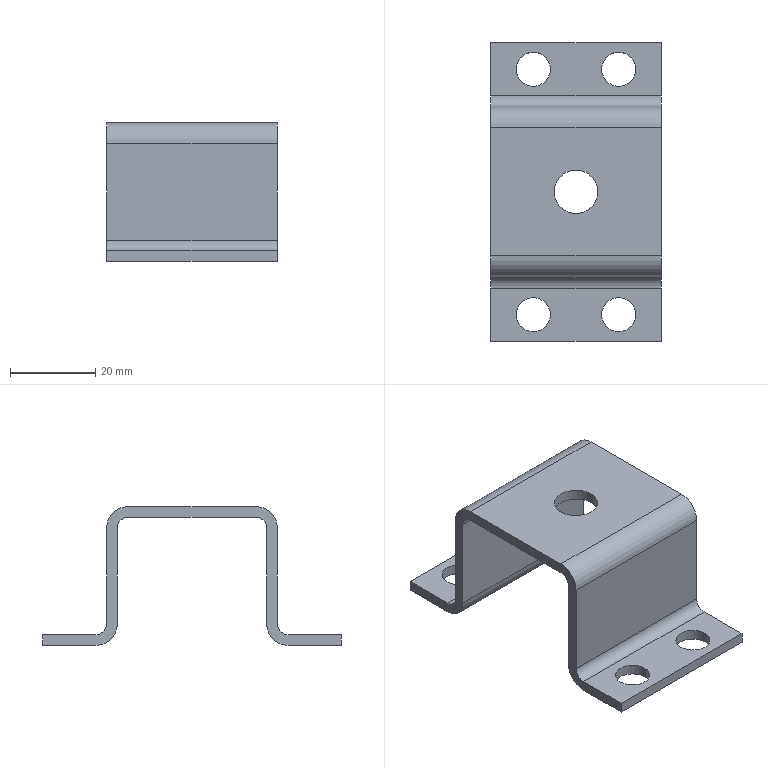Part | NX | features solid 2 | 1 solid | 32 faces | box 40 x 70 x 32.5 mm | volume 11649 mm3 | cylinder 18 | plane 14 | commonest cylinder face diameters 8 x8 5 x4 10 x4 10.2 x2
STEP:
#1=CARTESIAN_POINT('',(-932.,-1394.25,1257.));
#2=VERTEX_POINT('',#1);
#3=CARTESIAN_POINT('',(-932.,-1394.25,1259.5));
#4=VERTEX_POINT('',#3);
#5=CARTESIAN_POINT('',(-932.,-1394.25,1172.573));
#6=DIRECTION('',(0.,0.,1.));
#7=VECTOR('',#6,1000.);
#8=LINE('',#5,#7);
#9=EDGE_CURVE('',#2,#4,#8,.T.);
#10=ORIENTED_EDGE('',*,*,#9,.F.);
#11=CARTESIAN_POINT('',(-924.,-1394.25,1257.));
#12=VERTEX_POINT('',#11);
#13=CARTESIAN_POINT('',(-928.,-1394.25,1257.));
#14=DIRECTION('',(0.,0.,-1.));
#15=DIRECTION('',(0.,1.,0.));
#16=AXIS2_PLACEMENT_3D('',#13,#14,#15);
#17=CIRCLE('',#16,4.);
#18=EDGE_CURVE('',#2,#12,#17,.T.);
#19=ORIENTED_EDGE('',*,*,#18,.T.);
#20=CARTESIAN_POINT('',(-924.,-1394.25,1259.5));
#21=VERTEX_POINT('',#20);
#22=CARTESIAN_POINT('',(-924.,-1394.25,1172.573));
#23=DIRECTION('',(0.,0.,1.));
#24=VECTOR('',#23,1000.);
#25=LINE('',#22,#24);
#26=EDGE_CURVE('',#21,#12,#25,.F.);
#27=ORIENTED_EDGE('',*,*,#26,.F.);
#28=CARTESIAN_POINT('',(-928.,-1394.25,1259.5));
#29=DIRECTION('',(0.,0.,1.));
#30=DIRECTION('',(1.,0.,0.));
#31=AXIS2_PLACEMENT_3D('',#28,#29,#30);
#32=CIRCLE('',#31,4.);
#33=EDGE_CURVE('',#21,#4,#32,.T.);
#34=ORIENTED_EDGE('',*,*,#33,.T.);
#35=EDGE_LOOP('',(#10,#19,#27,#34));
#36=FACE_BOUND('',#35,.T.);
#37=CARTESIAN_POINT('',(-928.,-1394.25,1172.573));
#38=DIRECTION('',(0.,0.,1.));
#39=DIRECTION('',(1.,0.,0.));
#40=AXIS2_PLACEMENT_3D('',#37,#38,#39);
#41=CYLINDRICAL_SURFACE('',#40,4.);
#42=ADVANCED_FACE('',(#36),#41,.F.);
#43=CARTESIAN_POINT('',(-912.,-1394.25,1257.));
#44=VERTEX_POINT('',#43);
#45=CARTESIAN_POINT('',(-912.,-1394.25,1259.5));
#46=VERTEX_POINT('',#45);
#47=CARTESIAN_POINT('',(-912.,-1394.25,1172.573));
#48=DIRECTION('',(0.,0.,1.));
#49=VECTOR('',#48,1000.);
#50=LINE('',#47,#49);
#51=EDGE_CURVE('',#44,#46,#50,.T.);
#52=ORIENTED_EDGE('',*,*,#51,.F.);
#53=CARTESIAN_POINT('',(-904.,-1394.25,1257.));
#54=VERTEX_POINT('',#53);
#55=CARTESIAN_POINT('',(-908.,-1394.25,1257.));
#56=DIRECTION('',(0.,0.,-1.));
#57=DIRECTION('',(0.,1.,0.));
#58=AXIS2_PLACEMENT_3D('',#55,#56,#57);
#59=CIRCLE('',#58,4.);
#60=EDGE_CURVE('',#44,#54,#59,.T.);
#61=ORIENTED_EDGE('',*,*,#60,.T.);
#62=CARTESIAN_POINT('',(-904.,-1394.25,1259.5));
#63=VERTEX_POINT('',#62);
#64=CARTESIAN_POINT('',(-904.,-1394.25,1172.573));
#65=DIRECTION('',(0.,0.,1.));
#66=VECTOR('',#65,1000.);
#67=LINE('',#64,#66);
#68=EDGE_CURVE('',#63,#54,#67,.F.);
#69=ORIENTED_EDGE('',*,*,#68,.F.);
#70=CARTESIAN_POINT('',(-908.,-1394.25,1259.5));
#71=DIRECTION('',(0.,0.,1.));
#72=DIRECTION('',(1.,0.,0.));
#73=AXIS2_PLACEMENT_3D('',#70,#71,#72);
#74=CIRCLE('',#73,4.);
#75=EDGE_CURVE('',#63,#46,#74,.T.);
#76=ORIENTED_EDGE('',*,*,#75,.T.);
#77=EDGE_LOOP('',(#52,#61,#69,#76));
#78=FACE_BOUND('',#77,.T.);
#79=CARTESIAN_POINT('',(-908.,-1394.25,1172.573));
#80=DIRECTION('',(0.,0.,1.));
#81=DIRECTION('',(1.,0.,0.));
#82=AXIS2_PLACEMENT_3D('',#79,#80,#81);
#83=CYLINDRICAL_SURFACE('',#82,4.);
#84=ADVANCED_FACE('',(#78),#83,.F.);
#85=CARTESIAN_POINT('',(-912.,-1451.75,1257.));
#86=VERTEX_POINT('',#85);
#87=CARTESIAN_POINT('',(-912.,-1451.75,1259.5));
#88=VERTEX_POINT('',#87);
#89=CARTESIAN_POINT('',(-912.,-1451.75,1172.573));
#90=DIRECTION('',(0.,0.,1.));
#91=VECTOR('',#90,1000.);
#92=LINE('',#89,#91);
#93=EDGE_CURVE('',#86,#88,#92,.T.);
#94=ORIENTED_EDGE('',*,*,#93,.F.);
#95=CARTESIAN_POINT('',(-904.,-1451.75,1257.));
#96=VERTEX_POINT('',#95);
#97=CARTESIAN_POINT('',(-908.,-1451.75,1257.));
#98=DIRECTION('',(0.,0.,-1.));
#99=DIRECTION('',(-1.,0.,0.));
#100=AXIS2_PLACEMENT_3D('',#97,#98,#99);
#101=CIRCLE('',#100,4.);
#102=EDGE_CURVE('',#86,#96,#101,.T.);
#103=ORIENTED_EDGE('',*,*,#102,.T.);
#104=CARTESIAN_POINT('',(-904.,-1451.75,1259.5));
#105=VERTEX_POINT('',#104);
#106=CARTESIAN_POINT('',(-904.,-1451.75,1172.573));
#107=DIRECTION('',(0.,0.,1.));
#108=VECTOR('',#107,1000.);
#109=LINE('',#106,#108);
#110=EDGE_CURVE('',#105,#96,#109,.F.);
#111=ORIENTED_EDGE('',*,*,#110,.F.);
#112=CARTESIAN_POINT('',(-908.,-1451.75,1259.5));
#113=DIRECTION('',(0.,0.,1.));
#114=DIRECTION('',(1.,0.,0.));
#115=AXIS2_PLACEMENT_3D('',#112,#113,#114);
#116=CIRCLE('',#115,4.);
#117=EDGE_CURVE('',#105,#88,#116,.T.);
#118=ORIENTED_EDGE('',*,*,#117,.T.);
#119=EDGE_LOOP('',(#94,#103,#111,#118));
#120=FACE_BOUND('',#119,.T.);
#121=CARTESIAN_POINT('',(-908.,-1451.75,1172.573));
#122=DIRECTION('',(0.,0.,1.));
#123=DIRECTION('',(1.,0.,0.));
#124=AXIS2_PLACEMENT_3D('',#121,#122,#123);
#125=CYLINDRICAL_SURFACE('',#124,4.);
#126=ADVANCED_FACE('',(#120),#125,.F.);
#127=CARTESIAN_POINT('',(-932.,-1451.75,1257.));
#128=VERTEX_POINT('',#127);
#129=CARTESIAN_POINT('',(-932.,-1451.75,1259.5));
#130=VERTEX_POINT('',#129);
#131=CARTESIAN_POINT('',(-932.,-1451.75,1172.573));
#132=DIRECTION('',(0.,0.,1.));
#133=VECTOR('',#132,1000.);
#134=LINE('',#131,#133);
#135=EDGE_CURVE('',#128,#130,#134,.T.);
#136=ORIENTED_EDGE('',*,*,#135,.F.);
#137=CARTESIAN_POINT('',(-924.,-1451.75,1257.));
#138=VERTEX_POINT('',#137);
#139=CARTESIAN_POINT('',(-928.,-1451.75,1257.));
#140=DIRECTION('',(0.,0.,-1.));
#141=DIRECTION('',(-1.,0.,0.));
#142=AXIS2_PLACEMENT_3D('',#139,#140,#141);
#143=CIRCLE('',#142,4.);
#144=EDGE_CURVE('',#128,#138,#143,.T.);
#145=ORIENTED_EDGE('',*,*,#144,.T.);
#146=CARTESIAN_POINT('',(-924.,-1451.75,1259.5));
#147=VERTEX_POINT('',#146);
#148=CARTESIAN_POINT('',(-924.,-1451.75,1172.573));
#149=DIRECTION('',(0.,0.,1.));
#150=VECTOR('',#149,1000.);
#151=LINE('',#148,#150);
#152=EDGE_CURVE('',#147,#138,#151,.F.);
#153=ORIENTED_EDGE('',*,*,#152,.F.);
#154=CARTESIAN_POINT('',(-928.,-1451.75,1259.5));
#155=DIRECTION('',(0.,0.,1.));
#156=DIRECTION('',(1.,0.,0.));
#157=AXIS2_PLACEMENT_3D('',#154,#155,#156);
#158=CIRCLE('',#157,4.);
#159=EDGE_CURVE('',#147,#130,#158,.T.);
#160=ORIENTED_EDGE('',*,*,#159,.T.);
#161=EDGE_LOOP('',(#136,#145,#153,#160));
#162=FACE_BOUND('',#161,.T.);
#163=CARTESIAN_POINT('',(-928.,-1451.75,1172.573));
#164=DIRECTION('',(0.,0.,1.));
#165=DIRECTION('',(1.,0.,0.));
#166=AXIS2_PLACEMENT_3D('',#163,#164,#165);
#167=CYLINDRICAL_SURFACE('',#166,4.);
#168=ADVANCED_FACE('',(#162),#167,.F.);
#169=CARTESIAN_POINT('',(-923.1,-1423.,1289.5));
#170=VERTEX_POINT('',#169);
#171=CARTESIAN_POINT('',(-923.1,-1423.,1287.));
#172=VERTEX_POINT('',#171);
#173=CARTESIAN_POINT('',(-923.1,-1423.,1202.573));
#174=DIRECTION('',(0.,0.,1.));
#175=VECTOR('',#174,1000.);
#176=LINE('',#173,#175);
#177=EDGE_CURVE('',#170,#172,#176,.F.);
#178=ORIENTED_EDGE('',*,*,#177,.T.);
#179=CARTESIAN_POINT('',(-912.9,-1423.,1287.));
#180=VERTEX_POINT('',#179);
#181=CARTESIAN_POINT('',(-918.,-1423.,1287.));
#182=DIRECTION('',(0.,0.,-1.));
#183=DIRECTION('',(-1.,0.,0.));
#184=AXIS2_PLACEMENT_3D('',#181,#182,#183);
#185=CIRCLE('',#184,5.1);
#186=EDGE_CURVE('',#172,#180,#185,.T.);
#187=ORIENTED_EDGE('',*,*,#186,.T.);
#188=CARTESIAN_POINT('',(-912.9,-1423.,1289.5));
#189=VERTEX_POINT('',#188);
#190=CARTESIAN_POINT('',(-912.9,-1423.,1202.573));
#191=DIRECTION('',(0.,0.,1.));
#192=VECTOR('',#191,1000.);
#193=LINE('',#190,#192);
#194=EDGE_CURVE('',#180,#189,#193,.T.);
#195=ORIENTED_EDGE('',*,*,#194,.T.);
#196=CARTESIAN_POINT('',(-918.,-1423.,1289.5));
#197=DIRECTION('',(0.,0.,1.));
#198=DIRECTION('',(1.,0.,0.));
#199=AXIS2_PLACEMENT_3D('',#196,#197,#198);
#200=CIRCLE('',#199,5.1);
#201=EDGE_CURVE('',#189,#170,#200,.T.);
#202=ORIENTED_EDGE('',*,*,#201,.T.);
#203=EDGE_LOOP('',(#178,#187,#195,#202));
#204=FACE_BOUND('',#203,.T.);
#205=CARTESIAN_POINT('',(-918.,-1423.,1202.573));
#206=DIRECTION('',(0.,0.,1.));
#207=DIRECTION('',(1.,0.,0.));
#208=AXIS2_PLACEMENT_3D('',#205,#206,#207);
#209=CYLINDRICAL_SURFACE('',#208,5.1);
#210=ADVANCED_FACE('',(#204),#209,.F.);
#211=ORIENTED_EDGE('',*,*,#75,.F.);
#212=CARTESIAN_POINT('',(-908.,-1394.25,1259.5));
#213=DIRECTION('',(0.,0.,1.));
#214=DIRECTION('',(1.,0.,0.));
#215=AXIS2_PLACEMENT_3D('',#212,#213,#214);
#216=CIRCLE('',#215,4.);
#217=EDGE_CURVE('',#46,#63,#216,.T.);
#218=ORIENTED_EDGE('',*,*,#217,.F.);
#219=EDGE_LOOP('',(#211,#218));
#220=FACE_BOUND('',#219,.T.);
#221=ORIENTED_EDGE('',*,*,#33,.F.);
#222=CARTESIAN_POINT('',(-928.,-1394.25,1259.5));
#223=DIRECTION('',(0.,0.,1.));
#224=DIRECTION('',(1.,0.,0.));
#225=AXIS2_PLACEMENT_3D('',#222,#223,#224);
#226=CIRCLE('',#225,4.);
#227=EDGE_CURVE('',#4,#21,#226,.T.);
#228=ORIENTED_EDGE('',*,*,#227,.F.);
#229=EDGE_LOOP('',(#221,#228));
#230=FACE_BOUND('',#229,.T.);
#231=CARTESIAN_POINT('',(-898.,-1400.5,1259.5));
#232=VERTEX_POINT('',#231);
#233=CARTESIAN_POINT('',(-898.,-1388.,1259.5));
#234=VERTEX_POINT('',#233);
#235=CARTESIAN_POINT('',(-898.,-1403.,1259.5));
#236=DIRECTION('',(0.,1.,0.));
#237=VECTOR('',#236,1000.);
#238=LINE('',#235,#237);
#239=EDGE_CURVE('',#232,#234,#238,.T.);
#240=ORIENTED_EDGE('',*,*,#239,.T.);
#241=CARTESIAN_POINT('',(-938.,-1388.,1259.5));
#242=VERTEX_POINT('',#241);
#243=CARTESIAN_POINT('',(-938.,-1388.,1259.5));
#244=DIRECTION('',(1.,0.,0.));
#245=VECTOR('',#244,1000.);
#246=LINE('',#243,#245);
#247=EDGE_CURVE('',#242,#234,#246,.T.);
#248=ORIENTED_EDGE('',*,*,#247,.F.);
#249=CARTESIAN_POINT('',(-938.,-1400.5,1259.5));
#250=VERTEX_POINT('',#249);
#251=CARTESIAN_POINT('',(-938.,-1403.,1259.5));
#252=DIRECTION('',(0.,1.,0.));
#253=VECTOR('',#252,1000.);
#254=LINE('',#251,#253);
#255=EDGE_CURVE('',#250,#242,#254,.T.);
#256=ORIENTED_EDGE('',*,*,#255,.F.);
#257=CARTESIAN_POINT('',(-938.,-1400.5,1259.5));
#258=DIRECTION('',(1.,0.,0.));
#259=VECTOR('',#258,1000.);
#260=LINE('',#257,#259);
#261=EDGE_CURVE('',#250,#232,#260,.T.);
#262=ORIENTED_EDGE('',*,*,#261,.T.);
#263=EDGE_LOOP('',(#240,#248,#256,#262));
#264=FACE_BOUND('',#263,.T.);
#265=CARTESIAN_POINT('',(-938.,-1403.,1259.5));
#266=DIRECTION('',(0.,0.,-1.));
#267=DIRECTION('',(0.,-1.,0.));
#268=AXIS2_PLACEMENT_3D('',#265,#266,#267);
#269=PLANE('',#268);
#270=ADVANCED_FACE('',(#220,#230,#264),#269,.F.);
#271=CARTESIAN_POINT('',(-898.,-1403.,1262.));
#272=VERTEX_POINT('',#271);
#273=CARTESIAN_POINT('',(-898.,-1400.5,1262.));
#274=DIRECTION('',(1.,0.,0.));
#275=DIRECTION('',(0.,-1.,0.));
#276=AXIS2_PLACEMENT_3D('',#273,#274,#275);
#277=CIRCLE('',#276,2.5);
#278=EDGE_CURVE('',#272,#232,#277,.T.);
#279=ORIENTED_EDGE('',*,*,#278,.T.);
#280=ORIENTED_EDGE('',*,*,#261,.F.);
#281=CARTESIAN_POINT('',(-938.,-1403.,1262.));
#282=VERTEX_POINT('',#281);
#283=CARTESIAN_POINT('',(-938.,-1400.5,1262.));
#284=DIRECTION('',(1.,0.,0.));
#285=DIRECTION('',(0.,-1.,0.));
#286=AXIS2_PLACEMENT_3D('',#283,#284,#285);
#287=CIRCLE('',#286,2.5);
#288=EDGE_CURVE('',#282,#250,#287,.T.);
#289=ORIENTED_EDGE('',*,*,#288,.F.);
#290=CARTESIAN_POINT('',(-938.,-1403.,1262.));
#291=DIRECTION('',(1.,0.,0.));
#292=VECTOR('',#291,1000.);
#293=LINE('',#290,#292);
#294=EDGE_CURVE('',#282,#272,#293,.T.);
#295=ORIENTED_EDGE('',*,*,#294,.T.);
#296=EDGE_LOOP('',(#279,#280,#289,#295));
#297=FACE_BOUND('',#296,.T.);
#298=CARTESIAN_POINT('',(-938.,-1400.5,1262.));
#299=DIRECTION('',(1.,0.,0.));
#300=DIRECTION('',(0.,0.,-1.));
#301=AXIS2_PLACEMENT_3D('',#298,#299,#300);
#302=CYLINDRICAL_SURFACE('',#301,2.5);
#303=ADVANCED_FACE('',(#297),#302,.F.);
#304=CARTESIAN_POINT('',(-898.,-1403.,1284.5));
#305=VERTEX_POINT('',#304);
#306=CARTESIAN_POINT('',(-898.,-1403.,1289.5));
#307=DIRECTION('',(0.,0.,-1.));
#308=VECTOR('',#307,1000.);
#309=LINE('',#306,#308);
#310=EDGE_CURVE('',#305,#272,#309,.T.);
#311=ORIENTED_EDGE('',*,*,#310,.T.);
#312=ORIENTED_EDGE('',*,*,#294,.F.);
#313=CARTESIAN_POINT('',(-938.,-1403.,1284.5));
#314=VERTEX_POINT('',#313);
#315=CARTESIAN_POINT('',(-938.,-1403.,1289.5));
#316=DIRECTION('',(0.,0.,-1.));
#317=VECTOR('',#316,1000.);
#318=LINE('',#315,#317);
#319=EDGE_CURVE('',#314,#282,#318,.T.);
#320=ORIENTED_EDGE('',*,*,#319,.F.);
#321=CARTESIAN_POINT('',(-938.,-1403.,1284.5));
#322=DIRECTION('',(1.,0.,0.));
#323=VECTOR('',#322,1000.);
#324=LINE('',#321,#323);
#325=EDGE_CURVE('',#314,#305,#324,.T.);
#326=ORIENTED_EDGE('',*,*,#325,.T.);
#327=EDGE_LOOP('',(#311,#312,#320,#326));
#328=FACE_BOUND('',#327,.T.);
#329=CARTESIAN_POINT('',(-938.,-1403.,1289.5));
#330=DIRECTION('',(0.,-1.,0.));
#331=DIRECTION('',(0.,0.,-1.));
#332=AXIS2_PLACEMENT_3D('',#329,#330,#331);
#333=PLANE('',#332);
#334=ADVANCED_FACE('',(#328),#333,.F.);
#335=CARTESIAN_POINT('',(-898.,-1408.,1289.5));
#336=VERTEX_POINT('',#335);
#337=CARTESIAN_POINT('',(-898.,-1408.,1284.5));
#338=DIRECTION('',(-1.,0.,0.));
#339=DIRECTION('',(0.,1.,0.));
#340=AXIS2_PLACEMENT_3D('',#337,#338,#339);
#341=CIRCLE('',#340,5.);
#342=EDGE_CURVE('',#336,#305,#341,.T.);
#343=ORIENTED_EDGE('',*,*,#342,.T.);
#344=ORIENTED_EDGE('',*,*,#325,.F.);
#345=CARTESIAN_POINT('',(-938.,-1408.,1289.5));
#346=VERTEX_POINT('',#345);
#347=CARTESIAN_POINT('',(-938.,-1408.,1284.5));
#348=DIRECTION('',(-1.,0.,0.));
#349=DIRECTION('',(0.,1.,0.));
#350=AXIS2_PLACEMENT_3D('',#347,#348,#349);
#351=CIRCLE('',#350,5.);
#352=EDGE_CURVE('',#346,#314,#351,.T.);
#353=ORIENTED_EDGE('',*,*,#352,.F.);
#354=CARTESIAN_POINT('',(-938.,-1408.,1289.5));
#355=DIRECTION('',(1.,0.,0.));
#356=VECTOR('',#355,1000.);
#357=LINE('',#354,#356);
#358=EDGE_CURVE('',#346,#336,#357,.T.);
#359=ORIENTED_EDGE('',*,*,#358,.T.);
#360=EDGE_LOOP('',(#343,#344,#353,#359));
#361=FACE_BOUND('',#360,.T.);
#362=CARTESIAN_POINT('',(-938.,-1408.,1284.5));
#363=DIRECTION('',(1.,0.,0.));
#364=DIRECTION('',(0.,0.,-1.));
#365=AXIS2_PLACEMENT_3D('',#362,#363,#364);
#366=CYLINDRICAL_SURFACE('',#365,5.);
#367=ADVANCED_FACE('',(#361),#366,.T.);
#368=ORIENTED_EDGE('',*,*,#201,.F.);
#369=CARTESIAN_POINT('',(-918.,-1423.,1289.5));
#370=DIRECTION('',(0.,0.,1.));
#371=DIRECTION('',(1.,0.,0.));
#372=AXIS2_PLACEMENT_3D('',#369,#370,#371);
#373=CIRCLE('',#372,5.1);
#374=EDGE_CURVE('',#170,#189,#373,.T.);
#375=ORIENTED_EDGE('',*,*,#374,.F.);
#376=EDGE_LOOP('',(#368,#375));
#377=FACE_BOUND('',#376,.T.);
#378=CARTESIAN_POINT('',(-898.,-1438.,1289.5));
#379=VERTEX_POINT('',#378);
#380=CARTESIAN_POINT('',(-898.,-1443.,1289.5));
#381=DIRECTION('',(0.,1.,0.));
#382=VECTOR('',#381,1000.);
#383=LINE('',#380,#382);
#384=EDGE_CURVE('',#379,#336,#383,.T.);
#385=ORIENTED_EDGE('',*,*,#384,.T.);
#386=ORIENTED_EDGE('',*,*,#358,.F.);
#387=CARTESIAN_POINT('',(-938.,-1438.,1289.5));
#388=VERTEX_POINT('',#387);
#389=CARTESIAN_POINT('',(-938.,-1443.,1289.5));
#390=DIRECTION('',(0.,1.,0.));
#391=VECTOR('',#390,1000.);
#392=LINE('',#389,#391);
#393=EDGE_CURVE('',#388,#346,#392,.T.);
#394=ORIENTED_EDGE('',*,*,#393,.F.);
#395=CARTESIAN_POINT('',(-938.,-1438.,1289.5));
#396=DIRECTION('',(1.,0.,0.));
#397=VECTOR('',#396,1000.);
#398=LINE('',#395,#397);
#399=EDGE_CURVE('',#388,#379,#398,.T.);
#400=ORIENTED_EDGE('',*,*,#399,.T.);
#401=EDGE_LOOP('',(#385,#386,#394,#400));
#402=FACE_BOUND('',#401,.T.);
#403=CARTESIAN_POINT('',(-938.,-1443.,1289.5));
#404=DIRECTION('',(0.,0.,-1.));
#405=DIRECTION('',(0.,-1.,0.));
#406=AXIS2_PLACEMENT_3D('',#403,#404,#405);
#407=PLANE('',#406);
#408=ADVANCED_FACE('',(#377,#402),#407,.F.);
#409=CARTESIAN_POINT('',(-898.,-1443.,1284.5));
#410=VERTEX_POINT('',#409);
#411=CARTESIAN_POINT('',(-898.,-1438.,1284.5));
#412=DIRECTION('',(-1.,0.,0.));
#413=DIRECTION('',(0.,1.,0.));
#414=AXIS2_PLACEMENT_3D('',#411,#412,#413);
#415=CIRCLE('',#414,5.);
#416=EDGE_CURVE('',#410,#379,#415,.T.);
#417=ORIENTED_EDGE('',*,*,#416,.T.);
#418=ORIENTED_EDGE('',*,*,#399,.F.);
#419=CARTESIAN_POINT('',(-938.,-1443.,1284.5));
#420=VERTEX_POINT('',#419);
#421=CARTESIAN_POINT('',(-938.,-1438.,1284.5));
#422=DIRECTION('',(-1.,0.,0.));
#423=DIRECTION('',(0.,1.,0.));
#424=AXIS2_PLACEMENT_3D('',#421,#422,#423);
#425=CIRCLE('',#424,5.);
#426=EDGE_CURVE('',#420,#388,#425,.T.);
#427=ORIENTED_EDGE('',*,*,#426,.F.);
#428=CARTESIAN_POINT('',(-938.,-1443.,1284.5));
#429=DIRECTION('',(1.,0.,0.));
#430=VECTOR('',#429,1000.);
#431=LINE('',#428,#430);
#432=EDGE_CURVE('',#420,#410,#431,.T.);
#433=ORIENTED_EDGE('',*,*,#432,.T.);
#434=EDGE_LOOP('',(#417,#418,#427,#433));
#435=FACE_BOUND('',#434,.T.);
#436=CARTESIAN_POINT('',(-938.,-1438.,1284.5));
#437=DIRECTION('',(1.,0.,0.));
#438=DIRECTION('',(0.,0.,-1.));
#439=AXIS2_PLACEMENT_3D('',#436,#437,#438);
#440=CYLINDRICAL_SURFACE('',#439,5.);
#441=ADVANCED_FACE('',(#435),#440,.T.);
#442=CARTESIAN_POINT('',(-898.,-1443.,1262.));
#443=VERTEX_POINT('',#442);
#444=CARTESIAN_POINT('',(-898.,-1443.,1259.5));
#445=DIRECTION('',(0.,0.,1.));
#446=VECTOR('',#445,1000.);
#447=LINE('',#444,#446);
#448=EDGE_CURVE('',#443,#410,#447,.T.);
#449=ORIENTED_EDGE('',*,*,#448,.T.);
#450=ORIENTED_EDGE('',*,*,#432,.F.);
#451=CARTESIAN_POINT('',(-938.,-1443.,1262.));
#452=VERTEX_POINT('',#451);
#453=CARTESIAN_POINT('',(-938.,-1443.,1259.5));
#454=DIRECTION('',(0.,0.,1.));
#455=VECTOR('',#454,1000.);
#456=LINE('',#453,#455);
#457=EDGE_CURVE('',#452,#420,#456,.T.);
#458=ORIENTED_EDGE('',*,*,#457,.F.);
#459=CARTESIAN_POINT('',(-938.,-1443.,1262.));
#460=DIRECTION('',(1.,0.,0.));
#461=VECTOR('',#460,1000.);
#462=LINE('',#459,#461);
#463=EDGE_CURVE('',#452,#443,#462,.T.);
#464=ORIENTED_EDGE('',*,*,#463,.T.);
#465=EDGE_LOOP('',(#449,#450,#458,#464));
#466=FACE_BOUND('',#465,.T.);
#467=CARTESIAN_POINT('',(-938.,-1443.,1259.5));
#468=DIRECTION('',(0.,1.,0.));
#469=DIRECTION('',(0.,0.,-1.));
#470=AXIS2_PLACEMENT_3D('',#467,#468,#469);
#471=PLANE('',#470);
#472=ADVANCED_FACE('',(#466),#471,.F.);
#473=CARTESIAN_POINT('',(-898.,-1445.5,1259.5));
#474=VERTEX_POINT('',#473);
#475=CARTESIAN_POINT('',(-898.,-1445.5,1262.));
#476=DIRECTION('',(1.,0.,0.));
#477=DIRECTION('',(0.,-1.,0.));
#478=AXIS2_PLACEMENT_3D('',#475,#476,#477);
#479=CIRCLE('',#478,2.5);
#480=EDGE_CURVE('',#474,#443,#479,.T.);
#481=ORIENTED_EDGE('',*,*,#480,.T.);
#482=ORIENTED_EDGE('',*,*,#463,.F.);
#483=CARTESIAN_POINT('',(-938.,-1445.5,1259.5));
#484=VERTEX_POINT('',#483);
#485=CARTESIAN_POINT('',(-938.,-1445.5,1262.));
#486=DIRECTION('',(1.,0.,0.));
#487=DIRECTION('',(0.,-1.,0.));
#488=AXIS2_PLACEMENT_3D('',#485,#486,#487);
#489=CIRCLE('',#488,2.5);
#490=EDGE_CURVE('',#484,#452,#489,.T.);
#491=ORIENTED_EDGE('',*,*,#490,.F.);
#492=CARTESIAN_POINT('',(-938.,-1445.5,1259.5));
#493=DIRECTION('',(1.,0.,0.));
#494=VECTOR('',#493,1000.);
#495=LINE('',#492,#494);
#496=EDGE_CURVE('',#484,#474,#495,.T.);
#497=ORIENTED_EDGE('',*,*,#496,.T.);
#498=EDGE_LOOP('',(#481,#482,#491,#497));
#499=FACE_BOUND('',#498,.T.);
#500=CARTESIAN_POINT('',(-938.,-1445.5,1262.));
#501=DIRECTION('',(1.,0.,0.));
#502=DIRECTION('',(0.,0.,-1.));
#503=AXIS2_PLACEMENT_3D('',#500,#501,#502);
#504=CYLINDRICAL_SURFACE('',#503,2.5);
#505=ADVANCED_FACE('',(#499),#504,.F.);
#506=ORIENTED_EDGE('',*,*,#159,.F.);
#507=CARTESIAN_POINT('',(-928.,-1451.75,1259.5));
#508=DIRECTION('',(0.,0.,1.));
#509=DIRECTION('',(1.,0.,0.));
#510=AXIS2_PLACEMENT_3D('',#507,#508,#509);
#511=CIRCLE('',#510,4.);
#512=EDGE_CURVE('',#130,#147,#511,.T.);
#513=ORIENTED_EDGE('',*,*,#512,.F.);
#514=EDGE_LOOP('',(#506,#513));
#515=FACE_BOUND('',#514,.T.);
#516=ORIENTED_EDGE('',*,*,#117,.F.);
#517=CARTESIAN_POINT('',(-908.,-1451.75,1259.5));
#518=DIRECTION('',(0.,0.,1.));
#519=DIRECTION('',(1.,0.,0.));
#520=AXIS2_PLACEMENT_3D('',#517,#518,#519);
#521=CIRCLE('',#520,4.);
#522=EDGE_CURVE('',#88,#105,#521,.T.);
#523=ORIENTED_EDGE('',*,*,#522,.F.);
#524=EDGE_LOOP('',(#516,#523));
#525=FACE_BOUND('',#524,.T.);
#526=CARTESIAN_POINT('',(-898.,-1458.,1259.5));
#527=VERTEX_POINT('',#526);
#528=CARTESIAN_POINT('',(-898.,-1458.,1259.5));
#529=DIRECTION('',(0.,1.,0.));
#530=VECTOR('',#529,1000.);
#531=LINE('',#528,#530);
#532=EDGE_CURVE('',#527,#474,#531,.T.);
#533=ORIENTED_EDGE('',*,*,#532,.T.);
#534=ORIENTED_EDGE('',*,*,#496,.F.);
#535=CARTESIAN_POINT('',(-938.,-1458.,1259.5));
#536=VERTEX_POINT('',#535);
#537=CARTESIAN_POINT('',(-938.,-1458.,1259.5));
#538=DIRECTION('',(0.,1.,0.));
#539=VECTOR('',#538,1000.);
#540=LINE('',#537,#539);
#541=EDGE_CURVE('',#536,#484,#540,.T.);
#542=ORIENTED_EDGE('',*,*,#541,.F.);
#543=CARTESIAN_POINT('',(-938.,-1458.,1259.5));
#544=DIRECTION('',(1.,0.,0.));
#545=VECTOR('',#544,1000.);
#546=LINE('',#543,#545);
#547=EDGE_CURVE('',#536,#527,#546,.T.);
#548=ORIENTED_EDGE('',*,*,#547,.T.);
#549=EDGE_LOOP('',(#533,#534,#542,#548));
#550=FACE_BOUND('',#549,.T.);
#551=CARTESIAN_POINT('',(-938.,-1458.,1259.5));
#552=DIRECTION('',(0.,0.,-1.));
#553=DIRECTION('',(0.,-1.,0.));
#554=AXIS2_PLACEMENT_3D('',#551,#552,#553);
#555=PLANE('',#554);
#556=ADVANCED_FACE('',(#515,#525,#550),#555,.F.);
#557=CARTESIAN_POINT('',(-908.,-1394.25,1257.));
#558=DIRECTION('',(0.,0.,-1.));
#559=DIRECTION('',(0.,1.,0.));
#560=AXIS2_PLACEMENT_3D('',#557,#558,#559);
#561=CIRCLE('',#560,4.);
#562=EDGE_CURVE('',#54,#44,#561,.T.);
#563=ORIENTED_EDGE('',*,*,#562,.F.);
#564=ORIENTED_EDGE('',*,*,#60,.F.);
#565=EDGE_LOOP('',(#563,#564));
#566=FACE_BOUND('',#565,.T.);
#567=CARTESIAN_POINT('',(-928.,-1394.25,1257.));
#568=DIRECTION('',(0.,0.,-1.));
#569=DIRECTION('',(0.,1.,0.));
#570=AXIS2_PLACEMENT_3D('',#567,#568,#569);
#571=CIRCLE('',#570,4.);
#572=EDGE_CURVE('',#12,#2,#571,.T.);
#573=ORIENTED_EDGE('',*,*,#572,.F.);
#574=ORIENTED_EDGE('',*,*,#18,.F.);
#575=EDGE_LOOP('',(#573,#574));
#576=FACE_BOUND('',#575,.T.);
#577=CARTESIAN_POINT('',(-898.,-1400.5,1257.));
#578=VERTEX_POINT('',#577);
#579=CARTESIAN_POINT('',(-898.,-1388.,1257.));
#580=VERTEX_POINT('',#579);
#581=CARTESIAN_POINT('',(-898.,-1403.,1257.));
#582=DIRECTION('',(0.,1.,0.));
#583=VECTOR('',#582,1000.);
#584=LINE('',#581,#583);
#585=EDGE_CURVE('',#578,#580,#584,.T.);
#586=ORIENTED_EDGE('',*,*,#585,.F.);
#587=CARTESIAN_POINT('',(-938.,-1400.5,1257.));
#588=VERTEX_POINT('',#587);
#589=CARTESIAN_POINT('',(-938.,-1400.5,1257.));
#590=DIRECTION('',(1.,0.,0.));
#591=VECTOR('',#590,1000.);
#592=LINE('',#589,#591);
#593=EDGE_CURVE('',#588,#578,#592,.T.);
#594=ORIENTED_EDGE('',*,*,#593,.F.);
#595=CARTESIAN_POINT('',(-938.,-1388.,1257.));
#596=VERTEX_POINT('',#595);
#597=CARTESIAN_POINT('',(-938.,-1403.,1257.));
#598=DIRECTION('',(0.,1.,0.));
#599=VECTOR('',#598,1000.);
#600=LINE('',#597,#599);
#601=EDGE_CURVE('',#588,#596,#600,.T.);
#602=ORIENTED_EDGE('',*,*,#601,.T.);
#603=CARTESIAN_POINT('',(-938.,-1388.,1257.));
#604=DIRECTION('',(1.,0.,0.));
#605=VECTOR('',#604,1000.);
#606=LINE('',#603,#605);
#607=EDGE_CURVE('',#596,#580,#606,.T.);
#608=ORIENTED_EDGE('',*,*,#607,.T.);
#609=EDGE_LOOP('',(#586,#594,#602,#608));
#610=FACE_BOUND('',#609,.T.);
#611=CARTESIAN_POINT('',(-938.,-1403.,1257.));
#612=DIRECTION('',(0.,0.,-1.));
#613=DIRECTION('',(0.,-1.,0.));
#614=AXIS2_PLACEMENT_3D('',#611,#612,#613);
#615=PLANE('',#614);
#616=ADVANCED_FACE('',(#566,#576,#610),#615,.T.);
#617=CARTESIAN_POINT('',(-898.,-1405.5,1262.));
#618=VERTEX_POINT('',#617);
#619=CARTESIAN_POINT('',(-898.,-1400.5,1262.));
#620=DIRECTION('',(1.,0.,0.));
#621=DIRECTION('',(0.,0.,-1.));
#622=AXIS2_PLACEMENT_3D('',#619,#620,#621);
#623=CIRCLE('',#622,5.);
#624=EDGE_CURVE('',#618,#578,#623,.T.);
#625=ORIENTED_EDGE('',*,*,#624,.F.);
#626=CARTESIAN_POINT('',(-938.,-1405.5,1262.));
#627=VERTEX_POINT('',#626);
#628=CARTESIAN_POINT('',(-938.,-1405.5,1262.));
#629=DIRECTION('',(1.,0.,0.));
#630=VECTOR('',#629,1000.);
#631=LINE('',#628,#630);
#632=EDGE_CURVE('',#627,#618,#631,.T.);
#633=ORIENTED_EDGE('',*,*,#632,.F.);
#634=CARTESIAN_POINT('',(-938.,-1400.5,1262.));
#635=DIRECTION('',(1.,0.,0.));
#636=DIRECTION('',(0.,0.,-1.));
#637=AXIS2_PLACEMENT_3D('',#634,#635,#636);
#638=CIRCLE('',#637,5.);
#639=EDGE_CURVE('',#627,#588,#638,.T.);
#640=ORIENTED_EDGE('',*,*,#639,.T.);
#641=ORIENTED_EDGE('',*,*,#593,.T.);
#642=EDGE_LOOP('',(#625,#633,#640,#641));
#643=FACE_BOUND('',#642,.T.);
#644=CARTESIAN_POINT('',(-938.,-1400.5,1262.));
#645=DIRECTION('',(1.,0.,0.));
#646=DIRECTION('',(0.,0.,-1.));
#647=AXIS2_PLACEMENT_3D('',#644,#645,#646);
#648=CYLINDRICAL_SURFACE('',#647,5.);
#649=ADVANCED_FACE('',(#643),#648,.T.);
#650=CARTESIAN_POINT('',(-898.,-1405.5,1284.5));
#651=VERTEX_POINT('',#650);
#652=CARTESIAN_POINT('',(-898.,-1405.5,1289.5));
#653=DIRECTION('',(0.,0.,-1.));
#654=VECTOR('',#653,1000.);
#655=LINE('',#652,#654);
#656=EDGE_CURVE('',#651,#618,#655,.T.);
#657=ORIENTED_EDGE('',*,*,#656,.F.);
#658=CARTESIAN_POINT('',(-938.,-1405.5,1284.5));
#659=VERTEX_POINT('',#658);
#660=CARTESIAN_POINT('',(-938.,-1405.5,1284.5));
#661=DIRECTION('',(1.,0.,0.));
#662=VECTOR('',#661,1000.);
#663=LINE('',#660,#662);
#664=EDGE_CURVE('',#659,#651,#663,.T.);
#665=ORIENTED_EDGE('',*,*,#664,.F.);
#666=CARTESIAN_POINT('',(-938.,-1405.5,1289.5));
#667=DIRECTION('',(0.,0.,-1.));
#668=VECTOR('',#667,1000.);
#669=LINE('',#666,#668);
#670=EDGE_CURVE('',#659,#627,#669,.T.);
#671=ORIENTED_EDGE('',*,*,#670,.T.);
#672=ORIENTED_EDGE('',*,*,#632,.T.);
#673=EDGE_LOOP('',(#657,#665,#671,#672));
#674=FACE_BOUND('',#673,.T.);
#675=CARTESIAN_POINT('',(-938.,-1405.5,1289.5));
#676=DIRECTION('',(0.,-1.,0.));
#677=DIRECTION('',(0.,0.,-1.));
#678=AXIS2_PLACEMENT_3D('',#675,#676,#677);
#679=PLANE('',#678);
#680=ADVANCED_FACE('',(#674),#679,.T.);
#681=CARTESIAN_POINT('',(-898.,-1408.,1287.));
#682=VERTEX_POINT('',#681);
#683=CARTESIAN_POINT('',(-898.,-1408.,1284.5));
#684=DIRECTION('',(-1.,0.,0.));
#685=DIRECTION('',(0.,0.,-1.));
#686=AXIS2_PLACEMENT_3D('',#683,#684,#685);
#687=CIRCLE('',#686,2.5);
#688=EDGE_CURVE('',#682,#651,#687,.T.);
#689=ORIENTED_EDGE('',*,*,#688,.F.);
#690=CARTESIAN_POINT('',(-938.,-1408.,1287.));
#691=VERTEX_POINT('',#690);
#692=CARTESIAN_POINT('',(-938.,-1408.,1287.));
#693=DIRECTION('',(1.,0.,0.));
#694=VECTOR('',#693,1000.);
#695=LINE('',#692,#694);
#696=EDGE_CURVE('',#691,#682,#695,.T.);
#697=ORIENTED_EDGE('',*,*,#696,.F.);
#698=CARTESIAN_POINT('',(-938.,-1408.,1284.5));
#699=DIRECTION('',(-1.,0.,0.));
#700=DIRECTION('',(0.,0.,-1.));
#701=AXIS2_PLACEMENT_3D('',#698,#699,#700);
#702=CIRCLE('',#701,2.5);
#703=EDGE_CURVE('',#691,#659,#702,.T.);
#704=ORIENTED_EDGE('',*,*,#703,.T.);
#705=ORIENTED_EDGE('',*,*,#664,.T.);
#706=EDGE_LOOP('',(#689,#697,#704,#705));
#707=FACE_BOUND('',#706,.T.);
#708=CARTESIAN_POINT('',(-938.,-1408.,1284.5));
#709=DIRECTION('',(1.,0.,0.));
#710=DIRECTION('',(0.,0.,-1.));
#711=AXIS2_PLACEMENT_3D('',#708,#709,#710);
#712=CYLINDRICAL_SURFACE('',#711,2.5);
#713=ADVANCED_FACE('',(#707),#712,.F.);
#714=CARTESIAN_POINT('',(-918.,-1423.,1287.));
#715=DIRECTION('',(0.,0.,-1.));
#716=DIRECTION('',(-1.,0.,0.));
#717=AXIS2_PLACEMENT_3D('',#714,#715,#716);
#718=CIRCLE('',#717,5.1);
#719=EDGE_CURVE('',#180,#172,#718,.T.);
#720=ORIENTED_EDGE('',*,*,#719,.F.);
#721=ORIENTED_EDGE('',*,*,#186,.F.);
#722=EDGE_LOOP('',(#720,#721));
#723=FACE_BOUND('',#722,.T.);
#724=CARTESIAN_POINT('',(-898.,-1438.,1287.));
#725=VERTEX_POINT('',#724);
#726=CARTESIAN_POINT('',(-898.,-1443.,1287.));
#727=DIRECTION('',(0.,1.,0.));
#728=VECTOR('',#727,1000.);
#729=LINE('',#726,#728);
#730=EDGE_CURVE('',#725,#682,#729,.T.);
#731=ORIENTED_EDGE('',*,*,#730,.F.);
#732=CARTESIAN_POINT('',(-938.,-1438.,1287.));
#733=VERTEX_POINT('',#732);
#734=CARTESIAN_POINT('',(-938.,-1438.,1287.));
#735=DIRECTION('',(1.,0.,0.));
#736=VECTOR('',#735,1000.);
#737=LINE('',#734,#736);
#738=EDGE_CURVE('',#733,#725,#737,.T.);
#739=ORIENTED_EDGE('',*,*,#738,.F.);
#740=CARTESIAN_POINT('',(-938.,-1443.,1287.));
#741=DIRECTION('',(0.,1.,0.));
#742=VECTOR('',#741,1000.);
#743=LINE('',#740,#742);
#744=EDGE_CURVE('',#733,#691,#743,.T.);
#745=ORIENTED_EDGE('',*,*,#744,.T.);
#746=ORIENTED_EDGE('',*,*,#696,.T.);
#747=EDGE_LOOP('',(#731,#739,#745,#746));
#748=FACE_BOUND('',#747,.T.);
#749=CARTESIAN_POINT('',(-938.,-1443.,1287.));
#750=DIRECTION('',(0.,0.,-1.));
#751=DIRECTION('',(0.,-1.,0.));
#752=AXIS2_PLACEMENT_3D('',#749,#750,#751);
#753=PLANE('',#752);
#754=ADVANCED_FACE('',(#723,#748),#753,.T.);
#755=CARTESIAN_POINT('',(-898.,-1440.5,1284.5));
#756=VERTEX_POINT('',#755);
#757=CARTESIAN_POINT('',(-898.,-1438.,1284.5));
#758=DIRECTION('',(-1.,0.,0.));
#759=DIRECTION('',(0.,0.,-1.));
#760=AXIS2_PLACEMENT_3D('',#757,#758,#759);
#761=CIRCLE('',#760,2.5);
#762=EDGE_CURVE('',#756,#725,#761,.T.);
#763=ORIENTED_EDGE('',*,*,#762,.F.);
#764=CARTESIAN_POINT('',(-938.,-1440.5,1284.5));
#765=VERTEX_POINT('',#764);
#766=CARTESIAN_POINT('',(-938.,-1440.5,1284.5));
#767=DIRECTION('',(1.,0.,0.));
#768=VECTOR('',#767,1000.);
#769=LINE('',#766,#768);
#770=EDGE_CURVE('',#765,#756,#769,.T.);
#771=ORIENTED_EDGE('',*,*,#770,.F.);
#772=CARTESIAN_POINT('',(-938.,-1438.,1284.5));
#773=DIRECTION('',(-1.,0.,0.));
#774=DIRECTION('',(0.,0.,-1.));
#775=AXIS2_PLACEMENT_3D('',#772,#773,#774);
#776=CIRCLE('',#775,2.5);
#777=EDGE_CURVE('',#765,#733,#776,.T.);
#778=ORIENTED_EDGE('',*,*,#777,.T.);
#779=ORIENTED_EDGE('',*,*,#738,.T.);
#780=EDGE_LOOP('',(#763,#771,#778,#779));
#781=FACE_BOUND('',#780,.T.);
#782=CARTESIAN_POINT('',(-938.,-1438.,1284.5));
#783=DIRECTION('',(1.,0.,0.));
#784=DIRECTION('',(0.,0.,-1.));
#785=AXIS2_PLACEMENT_3D('',#782,#783,#784);
#786=CYLINDRICAL_SURFACE('',#785,2.5);
#787=ADVANCED_FACE('',(#781),#786,.F.);
#788=CARTESIAN_POINT('',(-898.,-1440.5,1262.));
#789=VERTEX_POINT('',#788);
#790=CARTESIAN_POINT('',(-898.,-1440.5,1259.5));
#791=DIRECTION('',(0.,0.,1.));
#792=VECTOR('',#791,1000.);
#793=LINE('',#790,#792);
#794=EDGE_CURVE('',#789,#756,#793,.T.);
#795=ORIENTED_EDGE('',*,*,#794,.F.);
#796=CARTESIAN_POINT('',(-938.,-1440.5,1262.));
#797=VERTEX_POINT('',#796);
#798=CARTESIAN_POINT('',(-938.,-1440.5,1262.));
#799=DIRECTION('',(1.,0.,0.));
#800=VECTOR('',#799,1000.);
#801=LINE('',#798,#800);
#802=EDGE_CURVE('',#797,#789,#801,.T.);
#803=ORIENTED_EDGE('',*,*,#802,.F.);
#804=CARTESIAN_POINT('',(-938.,-1440.5,1259.5));
#805=DIRECTION('',(0.,0.,1.));
#806=VECTOR('',#805,1000.);
#807=LINE('',#804,#806);
#808=EDGE_CURVE('',#797,#765,#807,.T.);
#809=ORIENTED_EDGE('',*,*,#808,.T.);
#810=ORIENTED_EDGE('',*,*,#770,.T.);
#811=EDGE_LOOP('',(#795,#803,#809,#810));
#812=FACE_BOUND('',#811,.T.);
#813=CARTESIAN_POINT('',(-938.,-1440.5,1259.5));
#814=DIRECTION('',(0.,1.,0.));
#815=DIRECTION('',(0.,0.,-1.));
#816=AXIS2_PLACEMENT_3D('',#813,#814,#815);
#817=PLANE('',#816);
#818=ADVANCED_FACE('',(#812),#817,.T.);
#819=CARTESIAN_POINT('',(-898.,-1445.5,1257.));
#820=VERTEX_POINT('',#819);
#821=CARTESIAN_POINT('',(-898.,-1445.5,1262.));
#822=DIRECTION('',(1.,0.,0.));
#823=DIRECTION('',(0.,0.,-1.));
#824=AXIS2_PLACEMENT_3D('',#821,#822,#823);
#825=CIRCLE('',#824,5.);
#826=EDGE_CURVE('',#820,#789,#825,.T.);
#827=ORIENTED_EDGE('',*,*,#826,.F.);
#828=CARTESIAN_POINT('',(-938.,-1445.5,1257.));
#829=VERTEX_POINT('',#828);
#830=CARTESIAN_POINT('',(-938.,-1445.5,1257.));
#831=DIRECTION('',(1.,0.,0.));
#832=VECTOR('',#831,1000.);
#833=LINE('',#830,#832);
#834=EDGE_CURVE('',#829,#820,#833,.T.);
#835=ORIENTED_EDGE('',*,*,#834,.F.);
#836=CARTESIAN_POINT('',(-938.,-1445.5,1262.));
#837=DIRECTION('',(1.,0.,0.));
#838=DIRECTION('',(0.,0.,-1.));
#839=AXIS2_PLACEMENT_3D('',#836,#837,#838);
#840=CIRCLE('',#839,5.);
#841=EDGE_CURVE('',#829,#797,#840,.T.);
#842=ORIENTED_EDGE('',*,*,#841,.T.);
#843=ORIENTED_EDGE('',*,*,#802,.T.);
#844=EDGE_LOOP('',(#827,#835,#842,#843));
#845=FACE_BOUND('',#844,.T.);
#846=CARTESIAN_POINT('',(-938.,-1445.5,1262.));
#847=DIRECTION('',(1.,0.,0.));
#848=DIRECTION('',(0.,0.,-1.));
#849=AXIS2_PLACEMENT_3D('',#846,#847,#848);
#850=CYLINDRICAL_SURFACE('',#849,5.);
#851=ADVANCED_FACE('',(#845),#850,.T.);
#852=CARTESIAN_POINT('',(-928.,-1451.75,1257.));
#853=DIRECTION('',(0.,0.,-1.));
#854=DIRECTION('',(-1.,0.,0.));
#855=AXIS2_PLACEMENT_3D('',#852,#853,#854);
#856=CIRCLE('',#855,4.);
#857=EDGE_CURVE('',#138,#128,#856,.T.);
#858=ORIENTED_EDGE('',*,*,#857,.F.);
#859=ORIENTED_EDGE('',*,*,#144,.F.);
#860=EDGE_LOOP('',(#858,#859));
#861=FACE_BOUND('',#860,.T.);
#862=CARTESIAN_POINT('',(-908.,-1451.75,1257.));
#863=DIRECTION('',(0.,0.,-1.));
#864=DIRECTION('',(-1.,0.,0.));
#865=AXIS2_PLACEMENT_3D('',#862,#863,#864);
#866=CIRCLE('',#865,4.);
#867=EDGE_CURVE('',#96,#86,#866,.T.);
#868=ORIENTED_EDGE('',*,*,#867,.F.);
#869=ORIENTED_EDGE('',*,*,#102,.F.);
#870=EDGE_LOOP('',(#868,#869));
#871=FACE_BOUND('',#870,.T.);
#872=CARTESIAN_POINT('',(-898.,-1458.,1257.));
#873=VERTEX_POINT('',#872);
#874=CARTESIAN_POINT('',(-898.,-1458.,1257.));
#875=DIRECTION('',(0.,1.,0.));
#876=VECTOR('',#875,1000.);
#877=LINE('',#874,#876);
#878=EDGE_CURVE('',#873,#820,#877,.T.);
#879=ORIENTED_EDGE('',*,*,#878,.F.);
#880=CARTESIAN_POINT('',(-938.,-1458.,1257.));
#881=VERTEX_POINT('',#880);
#882=CARTESIAN_POINT('',(-938.,-1458.,1257.));
#883=DIRECTION('',(1.,0.,0.));
#884=VECTOR('',#883,1000.);
#885=LINE('',#882,#884);
#886=EDGE_CURVE('',#881,#873,#885,.T.);
#887=ORIENTED_EDGE('',*,*,#886,.F.);
#888=CARTESIAN_POINT('',(-938.,-1458.,1257.));
#889=DIRECTION('',(0.,1.,0.));
#890=VECTOR('',#889,1000.);
#891=LINE('',#888,#890);
#892=EDGE_CURVE('',#881,#829,#891,.T.);
#893=ORIENTED_EDGE('',*,*,#892,.T.);
#894=ORIENTED_EDGE('',*,*,#834,.T.);
#895=EDGE_LOOP('',(#879,#887,#893,#894));
#896=FACE_BOUND('',#895,.T.);
#897=CARTESIAN_POINT('',(-938.,-1458.,1257.));
#898=DIRECTION('',(0.,0.,-1.));
#899=DIRECTION('',(0.,-1.,0.));
#900=AXIS2_PLACEMENT_3D('',#897,#898,#899);
#901=PLANE('',#900);
#902=ADVANCED_FACE('',(#861,#871,#896),#901,.T.);
#903=ORIENTED_EDGE('',*,*,#547,.F.);
#904=CARTESIAN_POINT('',(-938.,-1458.,1259.5));
#905=DIRECTION('',(0.,0.,-1.));
#906=VECTOR('',#905,1000.);
#907=LINE('',#904,#906);
#908=EDGE_CURVE('',#536,#881,#907,.T.);
#909=ORIENTED_EDGE('',*,*,#908,.T.);
#910=ORIENTED_EDGE('',*,*,#886,.T.);
#911=CARTESIAN_POINT('',(-898.,-1458.,1259.5));
#912=DIRECTION('',(0.,0.,-1.));
#913=VECTOR('',#912,1000.);
#914=LINE('',#911,#913);
#915=EDGE_CURVE('',#527,#873,#914,.T.);
#916=ORIENTED_EDGE('',*,*,#915,.F.);
#917=EDGE_LOOP('',(#903,#909,#910,#916));
#918=FACE_BOUND('',#917,.T.);
#919=CARTESIAN_POINT('',(-938.,-1458.,1259.5));
#920=DIRECTION('',(0.,1.,0.));
#921=DIRECTION('',(1.,0.,0.));
#922=AXIS2_PLACEMENT_3D('',#919,#920,#921);
#923=PLANE('',#922);
#924=ADVANCED_FACE('',(#918),#923,.F.);
#925=ORIENTED_EDGE('',*,*,#878,.T.);
#926=ORIENTED_EDGE('',*,*,#826,.T.);
#927=ORIENTED_EDGE('',*,*,#794,.T.);
#928=ORIENTED_EDGE('',*,*,#762,.T.);
#929=ORIENTED_EDGE('',*,*,#730,.T.);
#930=ORIENTED_EDGE('',*,*,#688,.T.);
#931=ORIENTED_EDGE('',*,*,#656,.T.);
#932=ORIENTED_EDGE('',*,*,#624,.T.);
#933=ORIENTED_EDGE('',*,*,#585,.T.);
#934=CARTESIAN_POINT('',(-898.,-1388.,1259.5));
#935=DIRECTION('',(0.,0.,-1.));
#936=VECTOR('',#935,1000.);
#937=LINE('',#934,#936);
#938=EDGE_CURVE('',#234,#580,#937,.T.);
#939=ORIENTED_EDGE('',*,*,#938,.F.);
#940=ORIENTED_EDGE('',*,*,#239,.F.);
#941=ORIENTED_EDGE('',*,*,#278,.F.);
#942=ORIENTED_EDGE('',*,*,#310,.F.);
#943=ORIENTED_EDGE('',*,*,#342,.F.);
#944=ORIENTED_EDGE('',*,*,#384,.F.);
#945=ORIENTED_EDGE('',*,*,#416,.F.);
#946=ORIENTED_EDGE('',*,*,#448,.F.);
#947=ORIENTED_EDGE('',*,*,#480,.F.);
#948=ORIENTED_EDGE('',*,*,#532,.F.);
#949=ORIENTED_EDGE('',*,*,#915,.T.);
#950=EDGE_LOOP('',(#925,#926,#927,#928,#929,#930,#931,#932,#933,#939,#940,#941,#942,#943,#944,#945,#946,#947,#948,#949));
#951=FACE_BOUND('',#950,.T.);
#952=CARTESIAN_POINT('',(-898.,-1458.,1259.5));
#953=DIRECTION('',(-1.,0.,0.));
#954=DIRECTION('',(0.,0.,1.));
#955=AXIS2_PLACEMENT_3D('',#952,#953,#954);
#956=PLANE('',#955);
#957=ADVANCED_FACE('',(#951),#956,.F.);
#958=CARTESIAN_POINT('',(-938.,-1388.,1259.5));
#959=DIRECTION('',(0.,0.,-1.));
#960=VECTOR('',#959,1000.);
#961=LINE('',#958,#960);
#962=EDGE_CURVE('',#242,#596,#961,.T.);
#963=ORIENTED_EDGE('',*,*,#962,.F.);
#964=ORIENTED_EDGE('',*,*,#247,.T.);
#965=ORIENTED_EDGE('',*,*,#938,.T.);
#966=ORIENTED_EDGE('',*,*,#607,.F.);
#967=EDGE_LOOP('',(#963,#964,#965,#966));
#968=FACE_BOUND('',#967,.T.);
#969=CARTESIAN_POINT('',(-938.,-1388.,1259.5));
#970=DIRECTION('',(0.,1.,0.));
#971=DIRECTION('',(0.,0.,-1.));
#972=AXIS2_PLACEMENT_3D('',#969,#970,#971);
#973=PLANE('',#972);
#974=ADVANCED_FACE('',(#968),#973,.T.);
#975=ORIENTED_EDGE('',*,*,#601,.F.);
#976=ORIENTED_EDGE('',*,*,#639,.F.);
#977=ORIENTED_EDGE('',*,*,#670,.F.);
#978=ORIENTED_EDGE('',*,*,#703,.F.);
#979=ORIENTED_EDGE('',*,*,#744,.F.);
#980=ORIENTED_EDGE('',*,*,#777,.F.);
#981=ORIENTED_EDGE('',*,*,#808,.F.);
#982=ORIENTED_EDGE('',*,*,#841,.F.);
#983=ORIENTED_EDGE('',*,*,#892,.F.);
#984=ORIENTED_EDGE('',*,*,#908,.F.);
#985=ORIENTED_EDGE('',*,*,#541,.T.);
#986=ORIENTED_EDGE('',*,*,#490,.T.);
#987=ORIENTED_EDGE('',*,*,#457,.T.);
#988=ORIENTED_EDGE('',*,*,#426,.T.);
#989=ORIENTED_EDGE('',*,*,#393,.T.);
#990=ORIENTED_EDGE('',*,*,#352,.T.);
#991=ORIENTED_EDGE('',*,*,#319,.T.);
#992=ORIENTED_EDGE('',*,*,#288,.T.);
#993=ORIENTED_EDGE('',*,*,#255,.T.);
#994=ORIENTED_EDGE('',*,*,#962,.T.);
#995=EDGE_LOOP('',(#975,#976,#977,#978,#979,#980,#981,#982,#983,#984,#985,#986,#987,#988,#989,#990,#991,#992,#993,#994));
#996=FACE_BOUND('',#995,.T.);
#997=CARTESIAN_POINT('',(-938.,-1403.,1259.5));
#998=DIRECTION('',(-1.,0.,0.));
#999=DIRECTION('',(0.,0.,1.));
#1000=AXIS2_PLACEMENT_3D('',#997,#998,#999);
#1001=PLANE('',#1000);
#1002=ADVANCED_FACE('',(#996),#1001,.T.);
#1003=ORIENTED_EDGE('',*,*,#719,.T.);
#1004=ORIENTED_EDGE('',*,*,#177,.F.);
#1005=ORIENTED_EDGE('',*,*,#374,.T.);
#1006=ORIENTED_EDGE('',*,*,#194,.F.);
#1007=EDGE_LOOP('',(#1003,#1004,#1005,#1006));
#1008=FACE_BOUND('',#1007,.T.);
#1009=CARTESIAN_POINT('',(-918.,-1423.,1202.573));
#1010=DIRECTION('',(0.,0.,1.));
#1011=DIRECTION('',(1.,0.,0.));
#1012=AXIS2_PLACEMENT_3D('',#1009,#1010,#1011);
#1013=CYLINDRICAL_SURFACE('',#1012,5.1);
#1014=ADVANCED_FACE('',(#1008),#1013,.F.);
#1015=ORIENTED_EDGE('',*,*,#857,.T.);
#1016=ORIENTED_EDGE('',*,*,#135,.T.);
#1017=ORIENTED_EDGE('',*,*,#512,.T.);
#1018=ORIENTED_EDGE('',*,*,#152,.T.);
#1019=EDGE_LOOP('',(#1015,#1016,#1017,#1018));
#1020=FACE_BOUND('',#1019,.T.);
#1021=CARTESIAN_POINT('',(-928.,-1451.75,1172.573));
#1022=DIRECTION('',(0.,0.,1.));
#1023=DIRECTION('',(1.,0.,0.));
#1024=AXIS2_PLACEMENT_3D('',#1021,#1022,#1023);
#1025=CYLINDRICAL_SURFACE('',#1024,4.);
#1026=ADVANCED_FACE('',(#1020),#1025,.F.);
#1027=ORIENTED_EDGE('',*,*,#867,.T.);
#1028=ORIENTED_EDGE('',*,*,#93,.T.);
#1029=ORIENTED_EDGE('',*,*,#522,.T.);
#1030=ORIENTED_EDGE('',*,*,#110,.T.);
#1031=EDGE_LOOP('',(#1027,#1028,#1029,#1030));
#1032=FACE_BOUND('',#1031,.T.);
#1033=CARTESIAN_POINT('',(-908.,-1451.75,1172.573));
#1034=DIRECTION('',(0.,0.,1.));
#1035=DIRECTION('',(1.,0.,0.));
#1036=AXIS2_PLACEMENT_3D('',#1033,#1034,#1035);
#1037=CYLINDRICAL_SURFACE('',#1036,4.);
#1038=ADVANCED_FACE('',(#1032),#1037,.F.);
#1039=ORIENTED_EDGE('',*,*,#562,.T.);
#1040=ORIENTED_EDGE('',*,*,#51,.T.);
#1041=ORIENTED_EDGE('',*,*,#217,.T.);
#1042=ORIENTED_EDGE('',*,*,#68,.T.);
#1043=EDGE_LOOP('',(#1039,#1040,#1041,#1042));
#1044=FACE_BOUND('',#1043,.T.);
#1045=CARTESIAN_POINT('',(-908.,-1394.25,1172.573));
#1046=DIRECTION('',(0.,0.,1.));
#1047=DIRECTION('',(1.,0.,0.));
#1048=AXIS2_PLACEMENT_3D('',#1045,#1046,#1047);
#1049=CYLINDRICAL_SURFACE('',#1048,4.);
#1050=ADVANCED_FACE('',(#1044),#1049,.F.);
#1051=ORIENTED_EDGE('',*,*,#572,.T.);
#1052=ORIENTED_EDGE('',*,*,#9,.T.);
#1053=ORIENTED_EDGE('',*,*,#227,.T.);
#1054=ORIENTED_EDGE('',*,*,#26,.T.);
#1055=EDGE_LOOP('',(#1051,#1052,#1053,#1054));
#1056=FACE_BOUND('',#1055,.T.);
#1057=CARTESIAN_POINT('',(-928.,-1394.25,1172.573));
#1058=DIRECTION('',(0.,0.,1.));
#1059=DIRECTION('',(1.,0.,0.));
#1060=AXIS2_PLACEMENT_3D('',#1057,#1058,#1059);
#1061=CYLINDRICAL_SURFACE('',#1060,4.);
#1062=ADVANCED_FACE('',(#1056),#1061,.F.);
#1063=CLOSED_SHELL('',(#42,#84,#126,#168,#210,#270,#303,#334,#367,#408,#441,#472,#505,#556,#616,#649,#680,#713,#754,#787,#818,#851,#902,#924,#957,#974,#1002,#1014,#1026,#1038,#1050,#1062));
#1064=MANIFOLD_SOLID_BREP('',#1063);
#1065=(LENGTH_UNIT()NAMED_UNIT(*)SI_UNIT(.MILLI.,.METRE.));
#1066=UNCERTAINTY_MEASURE_WITH_UNIT(LENGTH_MEASURE(0.00001),#1065,'','');
#1067=(NAMED_UNIT(*)PLANE_ANGLE_UNIT()SI_UNIT($,.RADIAN.));
#1068=(NAMED_UNIT(*)SI_UNIT($,.STERADIAN.)SOLID_ANGLE_UNIT());
#1069=(GEOMETRIC_REPRESENTATION_CONTEXT(3)GLOBAL_UNCERTAINTY_ASSIGNED_CONTEXT((#1066))GLOBAL_UNIT_ASSIGNED_CONTEXT((#1065,#1067,#1068))REPRESENTATION_CONTEXT('',''));
#1070=ADVANCED_BREP_SHAPE_REPRESENTATION('',(#1064),#1069);